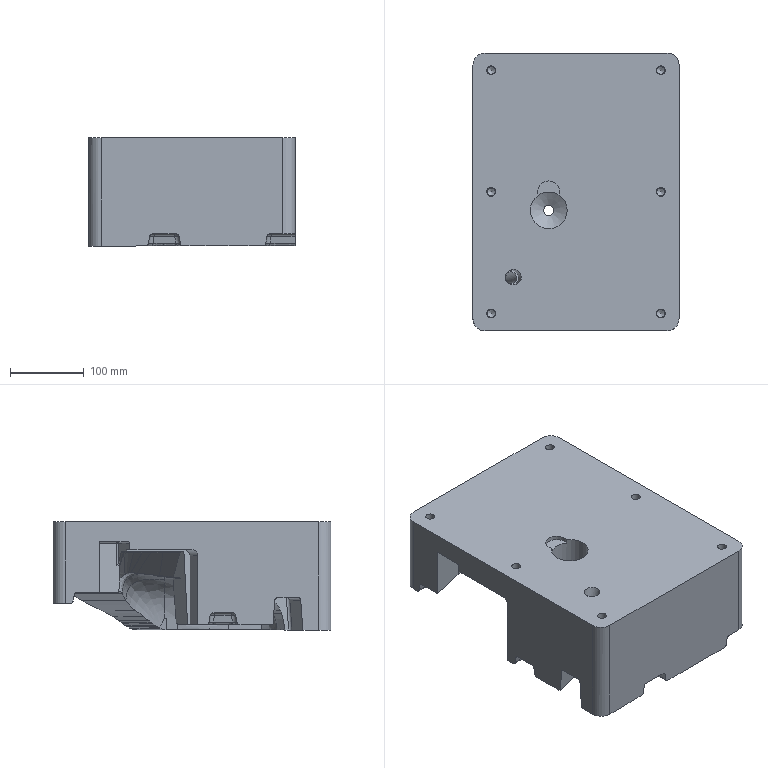Part | STEP file | 车灯-后视镜_id550_x_t | 1 solid | 357 faces | box 280 x 377 x 150.384 mm | volume 11421529 mm3 | spline 129 | plane 91 | cylinder 64 | other 64 | cone 7 | torus 1 | sphere 1 | commonest cylinder face diameters 8 x25 12 x16 10.4 x6 4 x4 33 x4 16 x3